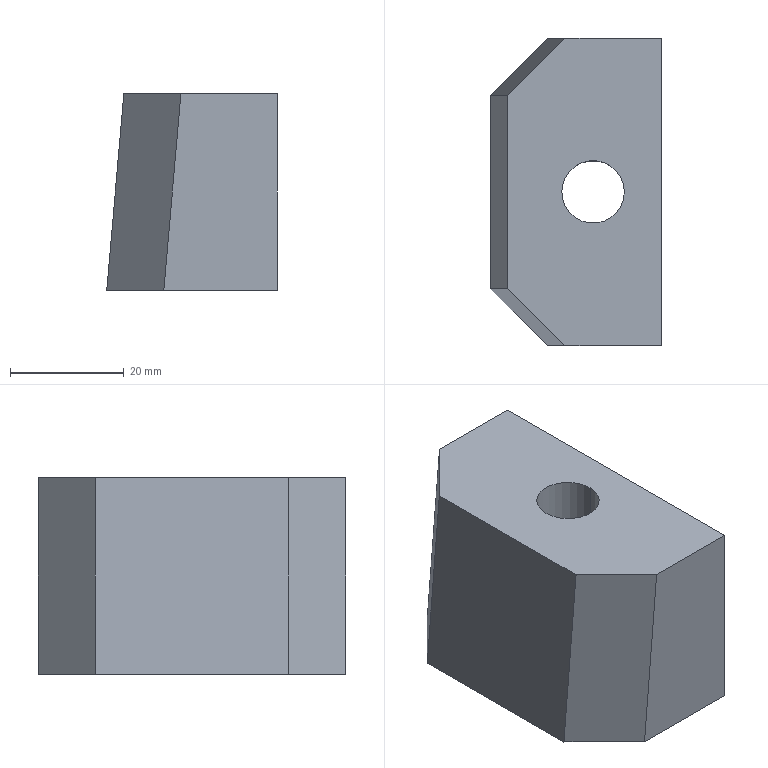Part | Creo | 1 solid | 78 faces | box 30 x 54 x 34.5 mm | volume 44422 mm3 | other 40 | plane 33 | cylinder 5 | commonest cylinder face diameters 11 x2 18 x2 1.666 x1